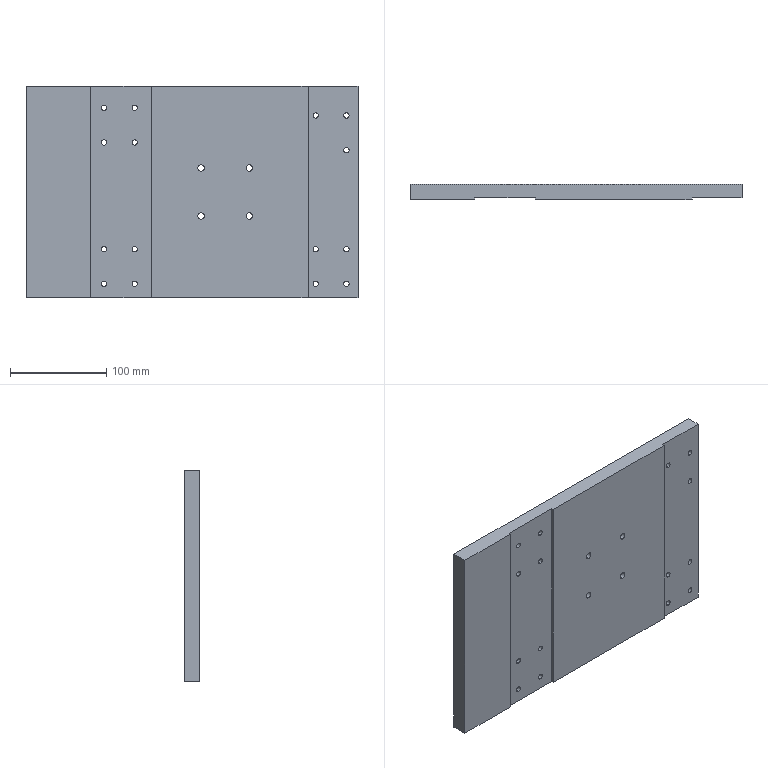Part | SolidWorks | features HoleWzd 2, Extrusion 1, ICE 1 | 1 solid | 95 faces | box 345 x 16 x 220 mm | volume 1151722 mm3 | cylinder 68 | plane 27 | commonest cylinder face diameters 5.5 x30 10 x30 6.8 x8